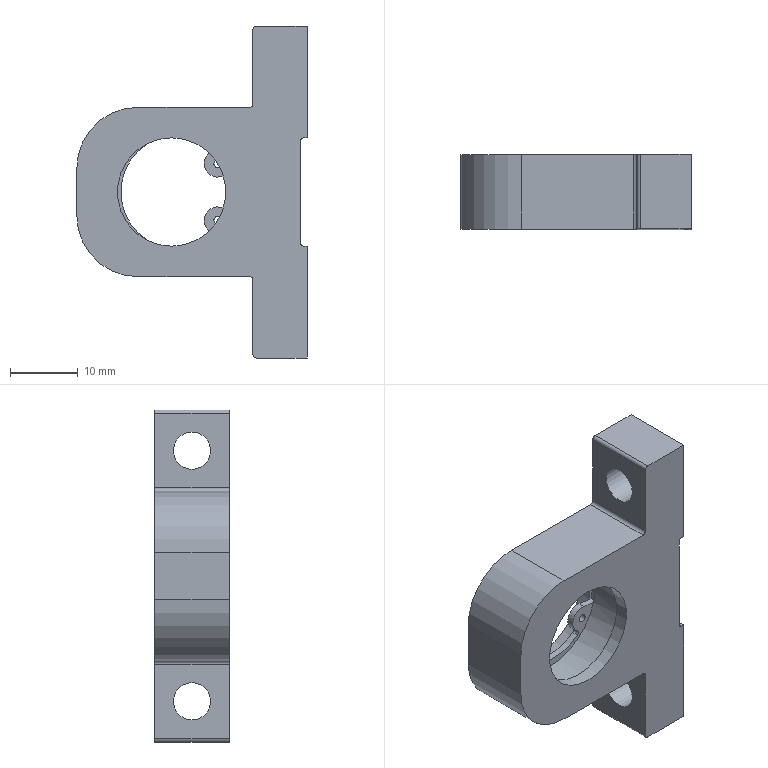Part | NX | features Housing_5003_021_C-BGHA698ZZ-20 2 | 1 solid | 42 faces | box 34 x 11 x 49 mm | volume 7650 mm3 | plane 21 | cylinder 21 | commonest cylinder face diameters 1 x8 1.2 x2 4.006 x2 5.5 x2 18 x2 19 x2
STEP:
#1=CARTESIAN_POINT('',(-207.617,-592.6,-107.974));
#2=VERTEX_POINT('',#1);
#3=CARTESIAN_POINT('',(-207.119,-592.6,-107.9));
#4=VERTEX_POINT('',#3);
#5=CARTESIAN_POINT('',(-209.667,-592.6,-108.281));
#6=DIRECTION('',(0.989,0.,0.1478));
#7=VECTOR('',#6,1000.);
#8=LINE('',#5,#7);
#9=EDGE_CURVE('',#2,#4,#8,.T.);
#10=ORIENTED_EDGE('',*,*,#9,.T.);
#11=CARTESIAN_POINT('',(-207.119,-592.6,-113.1));
#12=VERTEX_POINT('',#11);
#13=CARTESIAN_POINT('',(-216.775,-592.6,-110.5));
#14=DIRECTION('',(0.,-1.,0.));
#15=DIRECTION('',(0.,0.,1.));
#16=AXIS2_PLACEMENT_3D('',#13,#14,#15);
#17=CIRCLE('',#16,10.);
#18=EDGE_CURVE('',#12,#4,#17,.T.);
#19=ORIENTED_EDGE('',*,*,#18,.F.);
#20=CARTESIAN_POINT('',(-207.617,-592.6,-113.026));
#21=VERTEX_POINT('',#20);
#22=CARTESIAN_POINT('',(-209.667,-592.6,-112.719));
#23=DIRECTION('',(-0.989,0.,0.1478));
#24=VECTOR('',#23,1000.);
#25=LINE('',#22,#24);
#26=EDGE_CURVE('',#12,#21,#25,.T.);
#27=ORIENTED_EDGE('',*,*,#26,.T.);
#28=CARTESIAN_POINT('',(-216.775,-592.6,-110.5));
#29=DIRECTION('',(0.,-1.,0.));
#30=DIRECTION('',(0.,0.,1.));
#31=AXIS2_PLACEMENT_3D('',#28,#29,#30);
#32=CIRCLE('',#31,9.5);
#33=EDGE_CURVE('',#21,#2,#32,.T.);
#34=ORIENTED_EDGE('',*,*,#33,.T.);
#35=EDGE_LOOP('',(#10,#19,#27,#34));
#36=FACE_BOUND('',#35,.T.);
#37=CARTESIAN_POINT('',(-226.775,-592.6,-110.5));
#38=DIRECTION('',(0.,-1.,0.));
#39=DIRECTION('',(0.,0.,1.));
#40=AXIS2_PLACEMENT_3D('',#37,#38,#39);
#41=PLANE('',#40);
#42=ADVANCED_FACE('',(#36),#41,.F.);
#43=CARTESIAN_POINT('',(-207.119,-591.6,-107.9));
#44=VERTEX_POINT('',#43);
#45=CARTESIAN_POINT('',(-207.119,-592.6,-107.9));
#46=DIRECTION('',(0.,1.,0.));
#47=VECTOR('',#46,1000.);
#48=LINE('',#45,#47);
#49=EDGE_CURVE('',#4,#44,#48,.T.);
#50=ORIENTED_EDGE('',*,*,#49,.T.);
#51=CARTESIAN_POINT('',(-207.119,-591.6,-113.1));
#52=VERTEX_POINT('',#51);
#53=CARTESIAN_POINT('',(-216.775,-591.6,-110.5));
#54=DIRECTION('',(0.,-1.,0.));
#55=DIRECTION('',(0.,0.,1.));
#56=AXIS2_PLACEMENT_3D('',#53,#54,#55);
#57=CIRCLE('',#56,10.);
#58=EDGE_CURVE('',#52,#44,#57,.T.);
#59=ORIENTED_EDGE('',*,*,#58,.F.);
#60=CARTESIAN_POINT('',(-207.119,-592.6,-113.1));
#61=DIRECTION('',(0.,1.,0.));
#62=VECTOR('',#61,1000.);
#63=LINE('',#60,#62);
#64=EDGE_CURVE('',#12,#52,#63,.T.);
#65=ORIENTED_EDGE('',*,*,#64,.F.);
#66=ORIENTED_EDGE('',*,*,#18,.T.);
#67=EDGE_LOOP('',(#50,#59,#65,#66));
#68=FACE_BOUND('',#67,.T.);
#69=CARTESIAN_POINT('',(-216.775,-600.6,-110.5));
#70=DIRECTION('',(0.,-1.,0.));
#71=DIRECTION('',(0.,0.,1.));
#72=AXIS2_PLACEMENT_3D('',#69,#70,#71);
#73=CYLINDRICAL_SURFACE('',#72,10.);
#74=ADVANCED_FACE('',(#68),#73,.F.);
#75=CARTESIAN_POINT('',(-207.617,-591.6,-107.974));
#76=VERTEX_POINT('',#75);
#77=CARTESIAN_POINT('',(-226.237,-591.6,-110.757));
#78=DIRECTION('',(0.989,0.,0.1478));
#79=VECTOR('',#78,1000.);
#80=LINE('',#77,#79);
#81=EDGE_CURVE('',#76,#44,#80,.T.);
#82=ORIENTED_EDGE('',*,*,#81,.F.);
#83=CARTESIAN_POINT('',(-207.617,-591.6,-113.026));
#84=VERTEX_POINT('',#83);
#85=CARTESIAN_POINT('',(-216.775,-591.6,-110.5));
#86=DIRECTION('',(0.,-1.,0.));
#87=DIRECTION('',(0.,0.,1.));
#88=AXIS2_PLACEMENT_3D('',#85,#86,#87);
#89=CIRCLE('',#88,9.5);
#90=EDGE_CURVE('',#84,#76,#89,.T.);
#91=ORIENTED_EDGE('',*,*,#90,.F.);
#92=CARTESIAN_POINT('',(-209.667,-591.6,-112.719));
#93=DIRECTION('',(-0.989,0.,0.1478));
#94=VECTOR('',#93,1000.);
#95=LINE('',#92,#94);
#96=EDGE_CURVE('',#52,#84,#95,.T.);
#97=ORIENTED_EDGE('',*,*,#96,.F.);
#98=ORIENTED_EDGE('',*,*,#58,.T.);
#99=EDGE_LOOP('',(#82,#91,#97,#98));
#100=FACE_BOUND('',#99,.T.);
#101=CARTESIAN_POINT('',(-226.275,-591.6,-110.5));
#102=DIRECTION('',(0.,1.,0.));
#103=DIRECTION('',(0.,0.,-1.));
#104=AXIS2_PLACEMENT_3D('',#101,#102,#103);
#105=PLANE('',#104);
#106=ADVANCED_FACE('',(#100),#105,.F.);
#107=CARTESIAN_POINT('',(-196.775,-595.1,-126.25));
#108=VERTEX_POINT('',#107);
#109=CARTESIAN_POINT('',(-196.775,-595.1,-129.));
#110=DIRECTION('',(-1.,0.,0.));
#111=DIRECTION('',(0.,0.,1.));
#112=AXIS2_PLACEMENT_3D('',#109,#110,#111);
#113=CIRCLE('',#112,2.75);
#114=EDGE_CURVE('',#108,#108,#113,.T.);
#115=ORIENTED_EDGE('',*,*,#114,.T.);
#116=EDGE_LOOP('',(#115));
#117=FACE_BOUND('',#116,.T.);
#118=CARTESIAN_POINT('',(-196.775,-589.6,-118.5));
#119=VERTEX_POINT('',#118);
#120=CARTESIAN_POINT('',(-196.775,-589.6,-135.));
#121=VERTEX_POINT('',#120);
#122=CARTESIAN_POINT('',(-196.775,-589.6,-135.));
#123=DIRECTION('',(0.,0.,-1.));
#124=VECTOR('',#123,1000.);
#125=LINE('',#122,#124);
#126=EDGE_CURVE('',#119,#121,#125,.T.);
#127=ORIENTED_EDGE('',*,*,#126,.F.);
#128=CARTESIAN_POINT('',(-196.775,-600.6,-118.5));
#129=VERTEX_POINT('',#128);
#130=CARTESIAN_POINT('',(-196.775,-600.6,-118.5));
#131=DIRECTION('',(0.,1.,0.));
#132=VECTOR('',#131,1000.);
#133=LINE('',#130,#132);
#134=EDGE_CURVE('',#129,#119,#133,.T.);
#135=ORIENTED_EDGE('',*,*,#134,.F.);
#136=CARTESIAN_POINT('',(-196.775,-600.6,-135.));
#137=VERTEX_POINT('',#136);
#138=CARTESIAN_POINT('',(-196.775,-600.6,-135.));
#139=DIRECTION('',(0.,0.,-1.));
#140=VECTOR('',#139,1000.);
#141=LINE('',#138,#140);
#142=EDGE_CURVE('',#129,#137,#141,.T.);
#143=ORIENTED_EDGE('',*,*,#142,.T.);
#144=CARTESIAN_POINT('',(-196.775,-600.6,-135.));
#145=DIRECTION('',(0.,1.,0.));
#146=VECTOR('',#145,1000.);
#147=LINE('',#144,#146);
#148=EDGE_CURVE('',#137,#121,#147,.T.);
#149=ORIENTED_EDGE('',*,*,#148,.T.);
#150=EDGE_LOOP('',(#127,#135,#143,#149));
#151=FACE_BOUND('',#150,.T.);
#152=CARTESIAN_POINT('',(-196.775,-600.6,-135.));
#153=DIRECTION('',(1.,0.,0.));
#154=DIRECTION('',(0.,0.,-1.));
#155=AXIS2_PLACEMENT_3D('',#152,#153,#154);
#156=PLANE('',#155);
#157=ADVANCED_FACE('',(#117,#151),#156,.T.);
#158=CARTESIAN_POINT('',(-197.275,-589.6,-118.5));
#159=VERTEX_POINT('',#158);
#160=CARTESIAN_POINT('',(-197.275,-589.6,-118.5));
#161=DIRECTION('',(1.,0.,0.));
#162=VECTOR('',#161,1000.);
#163=LINE('',#160,#162);
#164=EDGE_CURVE('',#159,#119,#163,.T.);
#165=ORIENTED_EDGE('',*,*,#164,.F.);
#166=CARTESIAN_POINT('',(-197.275,-600.6,-118.5));
#167=VERTEX_POINT('',#166);
#168=CARTESIAN_POINT('',(-197.275,-600.6,-118.5));
#169=DIRECTION('',(0.,1.,0.));
#170=VECTOR('',#169,1000.);
#171=LINE('',#168,#170);
#172=EDGE_CURVE('',#167,#159,#171,.T.);
#173=ORIENTED_EDGE('',*,*,#172,.F.);
#174=CARTESIAN_POINT('',(-197.275,-600.6,-118.5));
#175=DIRECTION('',(1.,0.,0.));
#176=VECTOR('',#175,1000.);
#177=LINE('',#174,#176);
#178=EDGE_CURVE('',#167,#129,#177,.T.);
#179=ORIENTED_EDGE('',*,*,#178,.T.);
#180=ORIENTED_EDGE('',*,*,#134,.T.);
#181=EDGE_LOOP('',(#165,#173,#179,#180));
#182=FACE_BOUND('',#181,.T.);
#183=CARTESIAN_POINT('',(-197.275,-600.6,-118.5));
#184=DIRECTION('',(0.,0.,1.));
#185=DIRECTION('',(0.,1.,0.));
#186=AXIS2_PLACEMENT_3D('',#183,#184,#185);
#187=PLANE('',#186);
#188=ADVANCED_FACE('',(#182),#187,.T.);
#189=CARTESIAN_POINT('',(-197.775,-589.6,-118.));
#190=VERTEX_POINT('',#189);
#191=CARTESIAN_POINT('',(-197.275,-589.6,-118.));
#192=DIRECTION('',(0.,-1.,0.));
#193=DIRECTION('',(0.,0.,-1.));
#194=AXIS2_PLACEMENT_3D('',#191,#192,#193);
#195=CIRCLE('',#194,0.5);
#196=EDGE_CURVE('',#190,#159,#195,.T.);
#197=ORIENTED_EDGE('',*,*,#196,.F.);
#198=CARTESIAN_POINT('',(-197.775,-600.6,-118.));
#199=VERTEX_POINT('',#198);
#200=CARTESIAN_POINT('',(-197.775,-600.6,-118.));
#201=DIRECTION('',(0.,1.,0.));
#202=VECTOR('',#201,1000.);
#203=LINE('',#200,#202);
#204=EDGE_CURVE('',#199,#190,#203,.T.);
#205=ORIENTED_EDGE('',*,*,#204,.F.);
#206=CARTESIAN_POINT('',(-197.275,-600.6,-118.));
#207=DIRECTION('',(0.,-1.,0.));
#208=DIRECTION('',(0.,0.,-1.));
#209=AXIS2_PLACEMENT_3D('',#206,#207,#208);
#210=CIRCLE('',#209,0.5);
#211=EDGE_CURVE('',#199,#167,#210,.T.);
#212=ORIENTED_EDGE('',*,*,#211,.T.);
#213=ORIENTED_EDGE('',*,*,#172,.T.);
#214=EDGE_LOOP('',(#197,#205,#212,#213));
#215=FACE_BOUND('',#214,.T.);
#216=CARTESIAN_POINT('',(-197.275,-600.6,-118.));
#217=DIRECTION('',(0.,1.,0.));
#218=DIRECTION('',(0.,0.,-1.));
#219=AXIS2_PLACEMENT_3D('',#216,#217,#218);
#220=CYLINDRICAL_SURFACE('',#219,0.5);
#221=ADVANCED_FACE('',(#215),#220,.F.);
#222=CARTESIAN_POINT('',(-197.775,-589.6,-103.));
#223=VERTEX_POINT('',#222);
#224=CARTESIAN_POINT('',(-197.775,-589.6,-103.));
#225=DIRECTION('',(0.,0.,-1.));
#226=VECTOR('',#225,1000.);
#227=LINE('',#224,#226);
#228=EDGE_CURVE('',#223,#190,#227,.T.);
#229=ORIENTED_EDGE('',*,*,#228,.F.);
#230=CARTESIAN_POINT('',(-197.775,-600.6,-103.));
#231=VERTEX_POINT('',#230);
#232=CARTESIAN_POINT('',(-197.775,-600.6,-103.));
#233=DIRECTION('',(0.,1.,0.));
#234=VECTOR('',#233,1000.);
#235=LINE('',#232,#234);
#236=EDGE_CURVE('',#231,#223,#235,.T.);
#237=ORIENTED_EDGE('',*,*,#236,.F.);
#238=CARTESIAN_POINT('',(-197.775,-600.6,-103.));
#239=DIRECTION('',(0.,0.,-1.));
#240=VECTOR('',#239,1000.);
#241=LINE('',#238,#240);
#242=EDGE_CURVE('',#231,#199,#241,.T.);
#243=ORIENTED_EDGE('',*,*,#242,.T.);
#244=ORIENTED_EDGE('',*,*,#204,.T.);
#245=EDGE_LOOP('',(#229,#237,#243,#244));
#246=FACE_BOUND('',#245,.T.);
#247=CARTESIAN_POINT('',(-197.775,-600.6,-103.));
#248=DIRECTION('',(1.,0.,0.));
#249=DIRECTION('',(0.,0.,-1.));
#250=AXIS2_PLACEMENT_3D('',#247,#248,#249);
#251=PLANE('',#250);
#252=ADVANCED_FACE('',(#246),#251,.T.);
#253=CARTESIAN_POINT('',(-197.275,-589.6,-102.5));
#254=VERTEX_POINT('',#253);
#255=CARTESIAN_POINT('',(-197.275,-589.6,-103.));
#256=DIRECTION('',(0.,-1.,0.));
#257=DIRECTION('',(0.,0.,1.));
#258=AXIS2_PLACEMENT_3D('',#255,#256,#257);
#259=CIRCLE('',#258,0.5);
#260=EDGE_CURVE('',#254,#223,#259,.T.);
#261=ORIENTED_EDGE('',*,*,#260,.F.);
#262=CARTESIAN_POINT('',(-197.275,-600.6,-102.5));
#263=VERTEX_POINT('',#262);
#264=CARTESIAN_POINT('',(-197.275,-600.6,-102.5));
#265=DIRECTION('',(0.,1.,0.));
#266=VECTOR('',#265,1000.);
#267=LINE('',#264,#266);
#268=EDGE_CURVE('',#263,#254,#267,.T.);
#269=ORIENTED_EDGE('',*,*,#268,.F.);
#270=CARTESIAN_POINT('',(-197.275,-600.6,-103.));
#271=DIRECTION('',(0.,-1.,0.));
#272=DIRECTION('',(0.,0.,1.));
#273=AXIS2_PLACEMENT_3D('',#270,#271,#272);
#274=CIRCLE('',#273,0.5);
#275=EDGE_CURVE('',#263,#231,#274,.T.);
#276=ORIENTED_EDGE('',*,*,#275,.T.);
#277=ORIENTED_EDGE('',*,*,#236,.T.);
#278=EDGE_LOOP('',(#261,#269,#276,#277));
#279=FACE_BOUND('',#278,.T.);
#280=CARTESIAN_POINT('',(-197.275,-600.6,-103.));
#281=DIRECTION('',(0.,1.,0.));
#282=DIRECTION('',(0.,0.,-1.));
#283=AXIS2_PLACEMENT_3D('',#280,#281,#282);
#284=CYLINDRICAL_SURFACE('',#283,0.5);
#285=ADVANCED_FACE('',(#279),#284,.F.);
#286=CARTESIAN_POINT('',(-196.775,-589.6,-102.5));
#287=VERTEX_POINT('',#286);
#288=CARTESIAN_POINT('',(-197.275,-589.6,-102.5));
#289=DIRECTION('',(-1.,0.,0.));
#290=VECTOR('',#289,1000.);
#291=LINE('',#288,#290);
#292=EDGE_CURVE('',#287,#254,#291,.T.);
#293=ORIENTED_EDGE('',*,*,#292,.F.);
#294=CARTESIAN_POINT('',(-196.775,-600.6,-102.5));
#295=VERTEX_POINT('',#294);
#296=CARTESIAN_POINT('',(-196.775,-600.6,-102.5));
#297=DIRECTION('',(0.,1.,0.));
#298=VECTOR('',#297,1000.);
#299=LINE('',#296,#298);
#300=EDGE_CURVE('',#295,#287,#299,.T.);
#301=ORIENTED_EDGE('',*,*,#300,.F.);
#302=CARTESIAN_POINT('',(-197.275,-600.6,-102.5));
#303=DIRECTION('',(-1.,0.,0.));
#304=VECTOR('',#303,1000.);
#305=LINE('',#302,#304);
#306=EDGE_CURVE('',#295,#263,#305,.T.);
#307=ORIENTED_EDGE('',*,*,#306,.T.);
#308=ORIENTED_EDGE('',*,*,#268,.T.);
#309=EDGE_LOOP('',(#293,#301,#307,#308));
#310=FACE_BOUND('',#309,.T.);
#311=CARTESIAN_POINT('',(-197.275,-600.6,-102.5));
#312=DIRECTION('',(0.,0.,-1.));
#313=DIRECTION('',(0.,-1.,0.));
#314=AXIS2_PLACEMENT_3D('',#311,#312,#313);
#315=PLANE('',#314);
#316=ADVANCED_FACE('',(#310),#315,.T.);
#317=CARTESIAN_POINT('',(-196.775,-595.1,-89.25));
#318=VERTEX_POINT('',#317);
#319=CARTESIAN_POINT('',(-196.775,-595.1,-92.));
#320=DIRECTION('',(-1.,0.,0.));
#321=DIRECTION('',(0.,0.,1.));
#322=AXIS2_PLACEMENT_3D('',#319,#320,#321);
#323=CIRCLE('',#322,2.75);
#324=EDGE_CURVE('',#318,#318,#323,.T.);
#325=ORIENTED_EDGE('',*,*,#324,.T.);
#326=EDGE_LOOP('',(#325));
#327=FACE_BOUND('',#326,.T.);
#328=CARTESIAN_POINT('',(-196.775,-589.6,-86.));
#329=VERTEX_POINT('',#328);
#330=CARTESIAN_POINT('',(-196.775,-589.6,-102.5));
#331=DIRECTION('',(0.,0.,-1.));
#332=VECTOR('',#331,1000.);
#333=LINE('',#330,#332);
#334=EDGE_CURVE('',#329,#287,#333,.T.);
#335=ORIENTED_EDGE('',*,*,#334,.F.);
#336=CARTESIAN_POINT('',(-196.775,-600.6,-86.));
#337=VERTEX_POINT('',#336);
#338=CARTESIAN_POINT('',(-196.775,-600.6,-86.));
#339=DIRECTION('',(0.,1.,0.));
#340=VECTOR('',#339,1000.);
#341=LINE('',#338,#340);
#342=EDGE_CURVE('',#337,#329,#341,.T.);
#343=ORIENTED_EDGE('',*,*,#342,.F.);
#344=CARTESIAN_POINT('',(-196.775,-600.6,-102.5));
#345=DIRECTION('',(0.,0.,-1.));
#346=VECTOR('',#345,1000.);
#347=LINE('',#344,#346);
#348=EDGE_CURVE('',#337,#295,#347,.T.);
#349=ORIENTED_EDGE('',*,*,#348,.T.);
#350=ORIENTED_EDGE('',*,*,#300,.T.);
#351=EDGE_LOOP('',(#335,#343,#349,#350));
#352=FACE_BOUND('',#351,.T.);
#353=CARTESIAN_POINT('',(-196.775,-600.6,-102.5));
#354=DIRECTION('',(1.,0.,0.));
#355=DIRECTION('',(0.,0.,-1.));
#356=AXIS2_PLACEMENT_3D('',#353,#354,#355);
#357=PLANE('',#356);
#358=ADVANCED_FACE('',(#327,#352),#357,.T.);
#359=CARTESIAN_POINT('',(-204.275,-589.6,-86.));
#360=VERTEX_POINT('',#359);
#361=CARTESIAN_POINT('',(-196.775,-589.6,-86.));
#362=DIRECTION('',(1.,0.,0.));
#363=VECTOR('',#362,1000.);
#364=LINE('',#361,#363);
#365=EDGE_CURVE('',#360,#329,#364,.T.);
#366=ORIENTED_EDGE('',*,*,#365,.F.);
#367=CARTESIAN_POINT('',(-204.275,-600.6,-86.));
#368=VERTEX_POINT('',#367);
#369=CARTESIAN_POINT('',(-204.275,-600.6,-86.));
#370=DIRECTION('',(0.,1.,0.));
#371=VECTOR('',#370,1000.);
#372=LINE('',#369,#371);
#373=EDGE_CURVE('',#368,#360,#372,.T.);
#374=ORIENTED_EDGE('',*,*,#373,.F.);
#375=CARTESIAN_POINT('',(-196.775,-600.6,-86.));
#376=DIRECTION('',(1.,0.,0.));
#377=VECTOR('',#376,1000.);
#378=LINE('',#375,#377);
#379=EDGE_CURVE('',#368,#337,#378,.T.);
#380=ORIENTED_EDGE('',*,*,#379,.T.);
#381=ORIENTED_EDGE('',*,*,#342,.T.);
#382=EDGE_LOOP('',(#366,#374,#380,#381));
#383=FACE_BOUND('',#382,.T.);
#384=CARTESIAN_POINT('',(-196.775,-600.6,-86.));
#385=DIRECTION('',(0.,0.,1.));
#386=DIRECTION('',(0.,1.,0.));
#387=AXIS2_PLACEMENT_3D('',#384,#385,#386);
#388=PLANE('',#387);
#389=ADVANCED_FACE('',(#383),#388,.T.);
#390=CARTESIAN_POINT('',(-204.775,-589.6,-86.5));
#391=VERTEX_POINT('',#390);
#392=CARTESIAN_POINT('',(-204.275,-589.6,-86.5));
#393=DIRECTION('',(0.,1.,0.));
#394=DIRECTION('',(0.,0.,1.));
#395=AXIS2_PLACEMENT_3D('',#392,#393,#394);
#396=CIRCLE('',#395,0.5);
#397=EDGE_CURVE('',#391,#360,#396,.T.);
#398=ORIENTED_EDGE('',*,*,#397,.F.);
#399=CARTESIAN_POINT('',(-204.775,-600.6,-86.5));
#400=VERTEX_POINT('',#399);
#401=CARTESIAN_POINT('',(-204.775,-600.6,-86.5));
#402=DIRECTION('',(0.,1.,0.));
#403=VECTOR('',#402,1000.);
#404=LINE('',#401,#403);
#405=EDGE_CURVE('',#400,#391,#404,.T.);
#406=ORIENTED_EDGE('',*,*,#405,.F.);
#407=CARTESIAN_POINT('',(-204.275,-600.6,-86.5));
#408=DIRECTION('',(0.,1.,0.));
#409=DIRECTION('',(0.,0.,1.));
#410=AXIS2_PLACEMENT_3D('',#407,#408,#409);
#411=CIRCLE('',#410,0.5);
#412=EDGE_CURVE('',#400,#368,#411,.T.);
#413=ORIENTED_EDGE('',*,*,#412,.T.);
#414=ORIENTED_EDGE('',*,*,#373,.T.);
#415=EDGE_LOOP('',(#398,#406,#413,#414));
#416=FACE_BOUND('',#415,.T.);
#417=CARTESIAN_POINT('',(-204.275,-600.6,-86.5));
#418=DIRECTION('',(0.,1.,0.));
#419=DIRECTION('',(0.,0.,-1.));
#420=AXIS2_PLACEMENT_3D('',#417,#418,#419);
#421=CYLINDRICAL_SURFACE('',#420,0.5);
#422=ADVANCED_FACE('',(#416),#421,.T.);
#423=CARTESIAN_POINT('',(-204.775,-595.1,-89.25));
#424=VERTEX_POINT('',#423);
#425=CARTESIAN_POINT('',(-204.775,-595.1,-92.));
#426=DIRECTION('',(-1.,0.,0.));
#427=DIRECTION('',(0.,0.,1.));
#428=AXIS2_PLACEMENT_3D('',#425,#426,#427);
#429=CIRCLE('',#428,2.75);
#430=EDGE_CURVE('',#424,#424,#429,.T.);
#431=ORIENTED_EDGE('',*,*,#430,.F.);
#432=EDGE_LOOP('',(#431));
#433=FACE_BOUND('',#432,.T.);
#434=CARTESIAN_POINT('',(-204.775,-589.6,-97.5));
#435=VERTEX_POINT('',#434);
#436=CARTESIAN_POINT('',(-204.775,-589.6,-86.5));
#437=DIRECTION('',(0.,0.,1.));
#438=VECTOR('',#437,1000.);
#439=LINE('',#436,#438);
#440=EDGE_CURVE('',#435,#391,#439,.T.);
#441=ORIENTED_EDGE('',*,*,#440,.F.);
#442=CARTESIAN_POINT('',(-204.775,-600.6,-97.5));
#443=VERTEX_POINT('',#442);
#444=CARTESIAN_POINT('',(-204.775,-600.6,-97.5));
#445=DIRECTION('',(0.,1.,0.));
#446=VECTOR('',#445,1000.);
#447=LINE('',#444,#446);
#448=EDGE_CURVE('',#443,#435,#447,.T.);
#449=ORIENTED_EDGE('',*,*,#448,.F.);
#450=CARTESIAN_POINT('',(-204.775,-600.6,-86.5));
#451=DIRECTION('',(0.,0.,1.));
#452=VECTOR('',#451,1000.);
#453=LINE('',#450,#452);
#454=EDGE_CURVE('',#443,#400,#453,.T.);
#455=ORIENTED_EDGE('',*,*,#454,.T.);
#456=ORIENTED_EDGE('',*,*,#405,.T.);
#457=EDGE_LOOP('',(#441,#449,#455,#456));
#458=FACE_BOUND('',#457,.T.);
#459=CARTESIAN_POINT('',(-204.775,-600.6,-86.5));
#460=DIRECTION('',(-1.,0.,0.));
#461=DIRECTION('',(0.,0.,1.));
#462=AXIS2_PLACEMENT_3D('',#459,#460,#461);
#463=PLANE('',#462);
#464=ADVANCED_FACE('',(#433,#458),#463,.T.);
#465=CARTESIAN_POINT('',(-205.275,-589.6,-98.));
#466=VERTEX_POINT('',#465);
#467=CARTESIAN_POINT('',(-205.275,-589.6,-97.5));
#468=DIRECTION('',(0.,-1.,0.));
#469=DIRECTION('',(0.,0.,1.));
#470=AXIS2_PLACEMENT_3D('',#467,#468,#469);
#471=CIRCLE('',#470,0.5);
#472=EDGE_CURVE('',#466,#435,#471,.T.);
#473=ORIENTED_EDGE('',*,*,#472,.F.);
#474=CARTESIAN_POINT('',(-205.275,-600.6,-98.));
#475=VERTEX_POINT('',#474);
#476=CARTESIAN_POINT('',(-205.275,-600.6,-98.));
#477=DIRECTION('',(0.,1.,0.));
#478=VECTOR('',#477,1000.);
#479=LINE('',#476,#478);
#480=EDGE_CURVE('',#475,#466,#479,.T.);
#481=ORIENTED_EDGE('',*,*,#480,.F.);
#482=CARTESIAN_POINT('',(-205.275,-600.6,-97.5));
#483=DIRECTION('',(0.,-1.,0.));
#484=DIRECTION('',(0.,0.,1.));
#485=AXIS2_PLACEMENT_3D('',#482,#483,#484);
#486=CIRCLE('',#485,0.5);
#487=EDGE_CURVE('',#475,#443,#486,.T.);
#488=ORIENTED_EDGE('',*,*,#487,.T.);
#489=ORIENTED_EDGE('',*,*,#448,.T.);
#490=EDGE_LOOP('',(#473,#481,#488,#489));
#491=FACE_BOUND('',#490,.T.);
#492=CARTESIAN_POINT('',(-205.275,-600.6,-97.5));
#493=DIRECTION('',(0.,1.,0.));
#494=DIRECTION('',(0.,0.,-1.));
#495=AXIS2_PLACEMENT_3D('',#492,#493,#494);
#496=CYLINDRICAL_SURFACE('',#495,0.5);
#497=ADVANCED_FACE('',(#491),#496,.F.);
#498=CARTESIAN_POINT('',(-221.775,-589.6,-98.));
#499=VERTEX_POINT('',#498);
#500=CARTESIAN_POINT('',(-205.275,-589.6,-98.));
#501=DIRECTION('',(1.,0.,0.));
#502=VECTOR('',#501,1000.);
#503=LINE('',#500,#502);
#504=EDGE_CURVE('',#499,#466,#503,.T.);
#505=ORIENTED_EDGE('',*,*,#504,.F.);
#506=CARTESIAN_POINT('',(-221.775,-600.6,-98.));
#507=VERTEX_POINT('',#506);
#508=CARTESIAN_POINT('',(-221.775,-600.6,-98.));
#509=DIRECTION('',(0.,1.,0.));
#510=VECTOR('',#509,1000.);
#511=LINE('',#508,#510);
#512=EDGE_CURVE('',#507,#499,#511,.T.);
#513=ORIENTED_EDGE('',*,*,#512,.F.);
#514=CARTESIAN_POINT('',(-205.275,-600.6,-98.));
#515=DIRECTION('',(1.,0.,0.));
#516=VECTOR('',#515,1000.);
#517=LINE('',#514,#516);
#518=EDGE_CURVE('',#507,#475,#517,.T.);
#519=ORIENTED_EDGE('',*,*,#518,.T.);
#520=ORIENTED_EDGE('',*,*,#480,.T.);
#521=EDGE_LOOP('',(#505,#513,#519,#520));
#522=FACE_BOUND('',#521,.T.);
#523=CARTESIAN_POINT('',(-205.275,-600.6,-98.));
#524=DIRECTION('',(0.,0.,1.));
#525=DIRECTION('',(1.,0.,0.));
#526=AXIS2_PLACEMENT_3D('',#523,#524,#525);
#527=PLANE('',#526);
#528=ADVANCED_FACE('',(#522),#527,.T.);
#529=CARTESIAN_POINT('',(-230.775,-589.6,-107.));
#530=VERTEX_POINT('',#529);
#531=CARTESIAN_POINT('',(-221.775,-589.6,-107.));
#532=DIRECTION('',(0.,1.,0.));
#533=DIRECTION('',(0.,0.,1.));
#534=AXIS2_PLACEMENT_3D('',#531,#532,#533);
#535=CIRCLE('',#534,9.);
#536=EDGE_CURVE('',#530,#499,#535,.T.);
#537=ORIENTED_EDGE('',*,*,#536,.F.);
#538=CARTESIAN_POINT('',(-230.775,-600.6,-107.));
#539=VERTEX_POINT('',#538);
#540=CARTESIAN_POINT('',(-230.775,-600.6,-107.));
#541=DIRECTION('',(0.,1.,0.));
#542=VECTOR('',#541,1000.);
#543=LINE('',#540,#542);
#544=EDGE_CURVE('',#539,#530,#543,.T.);
#545=ORIENTED_EDGE('',*,*,#544,.F.);
#546=CARTESIAN_POINT('',(-221.775,-600.6,-107.));
#547=DIRECTION('',(0.,1.,0.));
#548=DIRECTION('',(0.,0.,1.));
#549=AXIS2_PLACEMENT_3D('',#546,#547,#548);
#550=CIRCLE('',#549,9.);
#551=EDGE_CURVE('',#539,#507,#550,.T.);
#552=ORIENTED_EDGE('',*,*,#551,.T.);
#553=ORIENTED_EDGE('',*,*,#512,.T.);
#554=EDGE_LOOP('',(#537,#545,#552,#553));
#555=FACE_BOUND('',#554,.T.);
#556=CARTESIAN_POINT('',(-221.775,-600.6,-107.));
#557=DIRECTION('',(0.,1.,0.));
#558=DIRECTION('',(0.,0.,-1.));
#559=AXIS2_PLACEMENT_3D('',#556,#557,#558);
#560=CYLINDRICAL_SURFACE('',#559,9.);
#561=ADVANCED_FACE('',(#555),#560,.T.);
#562=CARTESIAN_POINT('',(-230.775,-589.6,-114.));
#563=VERTEX_POINT('',#562);
#564=CARTESIAN_POINT('',(-230.775,-589.6,-107.));
#565=DIRECTION('',(0.,0.,1.));
#566=VECTOR('',#565,1000.);
#567=LINE('',#564,#566);
#568=EDGE_CURVE('',#563,#530,#567,.T.);
#569=ORIENTED_EDGE('',*,*,#568,.F.);
#570=CARTESIAN_POINT('',(-230.775,-600.6,-114.));
#571=VERTEX_POINT('',#570);
#572=CARTESIAN_POINT('',(-230.775,-600.6,-114.));
#573=DIRECTION('',(0.,1.,0.));
#574=VECTOR('',#573,1000.);
#575=LINE('',#572,#574);
#576=EDGE_CURVE('',#571,#563,#575,.T.);
#577=ORIENTED_EDGE('',*,*,#576,.F.);
#578=CARTESIAN_POINT('',(-230.775,-600.6,-107.));
#579=DIRECTION('',(0.,0.,1.));
#580=VECTOR('',#579,1000.);
#581=LINE('',#578,#580);
#582=EDGE_CURVE('',#571,#539,#581,.T.);
#583=ORIENTED_EDGE('',*,*,#582,.T.);
#584=ORIENTED_EDGE('',*,*,#544,.T.);
#585=EDGE_LOOP('',(#569,#577,#583,#584));
#586=FACE_BOUND('',#585,.T.);
#587=CARTESIAN_POINT('',(-230.775,-600.6,-107.));
#588=DIRECTION('',(-1.,0.,0.));
#589=DIRECTION('',(0.,0.,1.));
#590=AXIS2_PLACEMENT_3D('',#587,#588,#589);
#591=PLANE('',#590);
#592=ADVANCED_FACE('',(#586),#591,.T.);
#593=CARTESIAN_POINT('',(-221.775,-589.6,-123.));
#594=VERTEX_POINT('',#593);
#595=CARTESIAN_POINT('',(-221.775,-589.6,-114.));
#596=DIRECTION('',(0.,1.,0.));
#597=DIRECTION('',(0.,0.,-1.));
#598=AXIS2_PLACEMENT_3D('',#595,#596,#597);
#599=CIRCLE('',#598,9.);
#600=EDGE_CURVE('',#594,#563,#599,.T.);
#601=ORIENTED_EDGE('',*,*,#600,.F.);
#602=CARTESIAN_POINT('',(-221.775,-600.6,-123.));
#603=VERTEX_POINT('',#602);
#604=CARTESIAN_POINT('',(-221.775,-600.6,-123.));
#605=DIRECTION('',(0.,1.,0.));
#606=VECTOR('',#605,1000.);
#607=LINE('',#604,#606);
#608=EDGE_CURVE('',#603,#594,#607,.T.);
#609=ORIENTED_EDGE('',*,*,#608,.F.);
#610=CARTESIAN_POINT('',(-221.775,-600.6,-114.));
#611=DIRECTION('',(0.,1.,0.));
#612=DIRECTION('',(0.,0.,-1.));
#613=AXIS2_PLACEMENT_3D('',#610,#611,#612);
#614=CIRCLE('',#613,9.);
#615=EDGE_CURVE('',#603,#571,#614,.T.);
#616=ORIENTED_EDGE('',*,*,#615,.T.);
#617=ORIENTED_EDGE('',*,*,#576,.T.);
#618=EDGE_LOOP('',(#601,#609,#616,#617));
#619=FACE_BOUND('',#618,.T.);
#620=CARTESIAN_POINT('',(-221.775,-600.6,-114.));
#621=DIRECTION('',(0.,1.,0.));
#622=DIRECTION('',(0.,0.,-1.));
#623=AXIS2_PLACEMENT_3D('',#620,#621,#622);
#624=CYLINDRICAL_SURFACE('',#623,9.);
#625=ADVANCED_FACE('',(#619),#624,.T.);
#626=CARTESIAN_POINT('',(-205.275,-589.6,-123.));
#627=VERTEX_POINT('',#626);
#628=CARTESIAN_POINT('',(-221.775,-589.6,-123.));
#629=DIRECTION('',(-1.,0.,0.));
#630=VECTOR('',#629,1000.);
#631=LINE('',#628,#630);
#632=EDGE_CURVE('',#627,#594,#631,.T.);
#633=ORIENTED_EDGE('',*,*,#632,.F.);
#634=CARTESIAN_POINT('',(-205.275,-600.6,-123.));
#635=VERTEX_POINT('',#634);
#636=CARTESIAN_POINT('',(-205.275,-600.6,-123.));
#637=DIRECTION('',(0.,1.,0.));
#638=VECTOR('',#637,1000.);
#639=LINE('',#636,#638);
#640=EDGE_CURVE('',#635,#627,#639,.T.);
#641=ORIENTED_EDGE('',*,*,#640,.F.);
#642=CARTESIAN_POINT('',(-221.775,-600.6,-123.));
#643=DIRECTION('',(-1.,0.,0.));
#644=VECTOR('',#643,1000.);
#645=LINE('',#642,#644);
#646=EDGE_CURVE('',#635,#603,#645,.T.);
#647=ORIENTED_EDGE('',*,*,#646,.T.);
#648=ORIENTED_EDGE('',*,*,#608,.T.);
#649=EDGE_LOOP('',(#633,#641,#647,#648));
#650=FACE_BOUND('',#649,.T.);
#651=CARTESIAN_POINT('',(-221.775,-600.6,-123.));
#652=DIRECTION('',(0.,0.,-1.));
#653=DIRECTION('',(-1.,0.,0.));
#654=AXIS2_PLACEMENT_3D('',#651,#652,#653);
#655=PLANE('',#654);
#656=ADVANCED_FACE('',(#650),#655,.T.);
#657=CARTESIAN_POINT('',(-204.775,-589.6,-123.5));
#658=VERTEX_POINT('',#657);
#659=CARTESIAN_POINT('',(-205.275,-589.6,-123.5));
#660=DIRECTION('',(0.,-1.,0.));
#661=DIRECTION('',(0.,0.,1.));
#662=AXIS2_PLACEMENT_3D('',#659,#660,#661);
#663=CIRCLE('',#662,0.5);
#664=EDGE_CURVE('',#658,#627,#663,.T.);
#665=ORIENTED_EDGE('',*,*,#664,.F.);
#666=CARTESIAN_POINT('',(-204.775,-600.6,-123.5));
#667=VERTEX_POINT('',#666);
#668=CARTESIAN_POINT('',(-204.775,-600.6,-123.5));
#669=DIRECTION('',(0.,1.,0.));
#670=VECTOR('',#669,1000.);
#671=LINE('',#668,#670);
#672=EDGE_CURVE('',#667,#658,#671,.T.);
#673=ORIENTED_EDGE('',*,*,#672,.F.);
#674=CARTESIAN_POINT('',(-205.275,-600.6,-123.5));
#675=DIRECTION('',(0.,-1.,0.));
#676=DIRECTION('',(0.,0.,1.));
#677=AXIS2_PLACEMENT_3D('',#674,#675,#676);
#678=CIRCLE('',#677,0.5);
#679=EDGE_CURVE('',#667,#635,#678,.T.);
#680=ORIENTED_EDGE('',*,*,#679,.T.);
#681=ORIENTED_EDGE('',*,*,#640,.T.);
#682=EDGE_LOOP('',(#665,#673,#680,#681));
#683=FACE_BOUND('',#682,.T.);
#684=CARTESIAN_POINT('',(-205.275,-600.6,-123.5));
#685=DIRECTION('',(0.,1.,0.));
#686=DIRECTION('',(0.,0.,-1.));
#687=AXIS2_PLACEMENT_3D('',#684,#685,#686);
#688=CYLINDRICAL_SURFACE('',#687,0.5);
#689=ADVANCED_FACE('',(#683),#688,.F.);
#690=CARTESIAN_POINT('',(-204.775,-595.1,-126.25));
#691=VERTEX_POINT('',#690);
#692=CARTESIAN_POINT('',(-204.775,-595.1,-129.));
#693=DIRECTION('',(-1.,0.,0.));
#694=DIRECTION('',(0.,0.,1.));
#695=AXIS2_PLACEMENT_3D('',#692,#693,#694);
#696=CIRCLE('',#695,2.75);
#697=EDGE_CURVE('',#691,#691,#696,.T.);
#698=ORIENTED_EDGE('',*,*,#697,.F.);
#699=EDGE_LOOP('',(#698));
#700=FACE_BOUND('',#699,.T.);
#701=CARTESIAN_POINT('',(-204.775,-589.6,-134.5));
#702=VERTEX_POINT('',#701);
#703=CARTESIAN_POINT('',(-204.775,-589.6,-123.5));
#704=DIRECTION('',(0.,0.,1.));
#705=VECTOR('',#704,1000.);
#706=LINE('',#703,#705);
#707=EDGE_CURVE('',#702,#658,#706,.T.);
#708=ORIENTED_EDGE('',*,*,#707,.F.);
#709=CARTESIAN_POINT('',(-204.775,-600.6,-134.5));
#710=VERTEX_POINT('',#709);
#711=CARTESIAN_POINT('',(-204.775,-600.6,-134.5));
#712=DIRECTION('',(0.,1.,0.));
#713=VECTOR('',#712,1000.);
#714=LINE('',#711,#713);
#715=EDGE_CURVE('',#710,#702,#714,.T.);
#716=ORIENTED_EDGE('',*,*,#715,.F.);
#717=CARTESIAN_POINT('',(-204.775,-600.6,-123.5));
#718=DIRECTION('',(0.,0.,1.));
#719=VECTOR('',#718,1000.);
#720=LINE('',#717,#719);
#721=EDGE_CURVE('',#710,#667,#720,.T.);
#722=ORIENTED_EDGE('',*,*,#721,.T.);
#723=ORIENTED_EDGE('',*,*,#672,.T.);
#724=EDGE_LOOP('',(#708,#716,#722,#723));
#725=FACE_BOUND('',#724,.T.);
#726=CARTESIAN_POINT('',(-204.775,-600.6,-123.5));
#727=DIRECTION('',(-1.,0.,0.));
#728=DIRECTION('',(0.,0.,1.));
#729=AXIS2_PLACEMENT_3D('',#726,#727,#728);
#730=PLANE('',#729);
#731=ADVANCED_FACE('',(#700,#725),#730,.T.);
#732=CARTESIAN_POINT('',(-204.275,-589.6,-135.));
#733=VERTEX_POINT('',#732);
#734=CARTESIAN_POINT('',(-204.275,-589.6,-134.5));
#735=DIRECTION('',(0.,1.,0.));
#736=DIRECTION('',(0.,0.,-1.));
#737=AXIS2_PLACEMENT_3D('',#734,#735,#736);
#738=CIRCLE('',#737,0.5);
#739=EDGE_CURVE('',#733,#702,#738,.T.);
#740=ORIENTED_EDGE('',*,*,#739,.F.);
#741=CARTESIAN_POINT('',(-204.275,-600.6,-135.));
#742=VERTEX_POINT('',#741);
#743=CARTESIAN_POINT('',(-204.275,-600.6,-135.));
#744=DIRECTION('',(0.,1.,0.));
#745=VECTOR('',#744,1000.);
#746=LINE('',#743,#745);
#747=EDGE_CURVE('',#742,#733,#746,.T.);
#748=ORIENTED_EDGE('',*,*,#747,.F.);
#749=CARTESIAN_POINT('',(-204.275,-600.6,-134.5));
#750=DIRECTION('',(0.,1.,0.));
#751=DIRECTION('',(0.,0.,-1.));
#752=AXIS2_PLACEMENT_3D('',#749,#750,#751);
#753=CIRCLE('',#752,0.5);
#754=EDGE_CURVE('',#742,#710,#753,.T.);
#755=ORIENTED_EDGE('',*,*,#754,.T.);
#756=ORIENTED_EDGE('',*,*,#715,.T.);
#757=EDGE_LOOP('',(#740,#748,#755,#756));
#758=FACE_BOUND('',#757,.T.);
#759=CARTESIAN_POINT('',(-204.275,-600.6,-134.5));
#760=DIRECTION('',(0.,1.,0.));
#761=DIRECTION('',(0.,0.,-1.));
#762=AXIS2_PLACEMENT_3D('',#759,#760,#761);
#763=CYLINDRICAL_SURFACE('',#762,0.5);
#764=ADVANCED_FACE('',(#758),#763,.T.);
#765=CARTESIAN_POINT('',(-204.275,-589.6,-135.));
#766=DIRECTION('',(-1.,0.,0.));
#767=VECTOR('',#766,1000.);
#768=LINE('',#765,#767);
#769=EDGE_CURVE('',#121,#733,#768,.T.);
#770=ORIENTED_EDGE('',*,*,#769,.F.);
#771=ORIENTED_EDGE('',*,*,#148,.F.);
#772=CARTESIAN_POINT('',(-204.275,-600.6,-135.));
#773=DIRECTION('',(-1.,0.,0.));
#774=VECTOR('',#773,1000.);
#775=LINE('',#772,#774);
#776=EDGE_CURVE('',#137,#742,#775,.T.);
#777=ORIENTED_EDGE('',*,*,#776,.T.);
#778=ORIENTED_EDGE('',*,*,#747,.T.);
#779=EDGE_LOOP('',(#770,#771,#777,#778));
#780=FACE_BOUND('',#779,.T.);
#781=CARTESIAN_POINT('',(-204.275,-600.6,-135.));
#782=DIRECTION('',(0.,0.,-1.));
#783=DIRECTION('',(0.,-1.,0.));
#784=AXIS2_PLACEMENT_3D('',#781,#782,#783);
#785=PLANE('',#784);
#786=ADVANCED_FACE('',(#780),#785,.T.);
#787=CARTESIAN_POINT('',(-216.775,-600.6,-102.5));
#788=VERTEX_POINT('',#787);
#789=CARTESIAN_POINT('',(-216.775,-600.6,-110.5));
#790=DIRECTION('',(0.,-1.,0.));
#791=DIRECTION('',(0.,0.,1.));
#792=AXIS2_PLACEMENT_3D('',#789,#790,#791);
#793=CIRCLE('',#792,8.);
#794=EDGE_CURVE('',#788,#788,#793,.T.);
#795=ORIENTED_EDGE('',*,*,#794,.F.);
#796=EDGE_LOOP('',(#795));
#797=FACE_BOUND('',#796,.T.);
#798=ORIENTED_EDGE('',*,*,#142,.F.);
#799=ORIENTED_EDGE('',*,*,#178,.F.);
#800=ORIENTED_EDGE('',*,*,#211,.F.);
#801=ORIENTED_EDGE('',*,*,#242,.F.);
#802=ORIENTED_EDGE('',*,*,#275,.F.);
#803=ORIENTED_EDGE('',*,*,#306,.F.);
#804=ORIENTED_EDGE('',*,*,#348,.F.);
#805=ORIENTED_EDGE('',*,*,#379,.F.);
#806=ORIENTED_EDGE('',*,*,#412,.F.);
#807=ORIENTED_EDGE('',*,*,#454,.F.);
#808=ORIENTED_EDGE('',*,*,#487,.F.);
#809=ORIENTED_EDGE('',*,*,#518,.F.);
#810=ORIENTED_EDGE('',*,*,#551,.F.);
#811=ORIENTED_EDGE('',*,*,#582,.F.);
#812=ORIENTED_EDGE('',*,*,#615,.F.);
#813=ORIENTED_EDGE('',*,*,#646,.F.);
#814=ORIENTED_EDGE('',*,*,#679,.F.);
#815=ORIENTED_EDGE('',*,*,#721,.F.);
#816=ORIENTED_EDGE('',*,*,#754,.F.);
#817=ORIENTED_EDGE('',*,*,#776,.F.);
#818=EDGE_LOOP('',(#798,#799,#800,#801,#802,#803,#804,#805,#806,#807,#808,#809,#810,#811,#812,#813,#814,#815,#816,#817));
#819=FACE_BOUND('',#818,.T.);
#820=CARTESIAN_POINT('',(-197.275,-600.6,-118.));
#821=DIRECTION('',(0.,1.,0.));
#822=DIRECTION('',(0.,0.,-1.));
#823=AXIS2_PLACEMENT_3D('',#820,#821,#822);
#824=PLANE('',#823);
#825=ADVANCED_FACE('',(#797,#819),#824,.F.);
#826=CARTESIAN_POINT('',(-216.775,-589.6,-101.));
#827=VERTEX_POINT('',#826);
#828=CARTESIAN_POINT('',(-216.775,-589.6,-110.5));
#829=DIRECTION('',(0.,-1.,0.));
#830=DIRECTION('',(0.,0.,1.));
#831=AXIS2_PLACEMENT_3D('',#828,#829,#830);
#832=CIRCLE('',#831,9.5);
#833=EDGE_CURVE('',#827,#827,#832,.T.);
#834=ORIENTED_EDGE('',*,*,#833,.T.);
#835=EDGE_LOOP('',(#834));
#836=FACE_BOUND('',#835,.T.);
#837=ORIENTED_EDGE('',*,*,#126,.T.);
#838=ORIENTED_EDGE('',*,*,#769,.T.);
#839=ORIENTED_EDGE('',*,*,#739,.T.);
#840=ORIENTED_EDGE('',*,*,#707,.T.);
#841=ORIENTED_EDGE('',*,*,#664,.T.);
#842=ORIENTED_EDGE('',*,*,#632,.T.);
#843=ORIENTED_EDGE('',*,*,#600,.T.);
#844=ORIENTED_EDGE('',*,*,#568,.T.);
#845=ORIENTED_EDGE('',*,*,#536,.T.);
#846=ORIENTED_EDGE('',*,*,#504,.T.);
#847=ORIENTED_EDGE('',*,*,#472,.T.);
#848=ORIENTED_EDGE('',*,*,#440,.T.);
#849=ORIENTED_EDGE('',*,*,#397,.T.);
#850=ORIENTED_EDGE('',*,*,#365,.T.);
#851=ORIENTED_EDGE('',*,*,#334,.T.);
#852=ORIENTED_EDGE('',*,*,#292,.T.);
#853=ORIENTED_EDGE('',*,*,#260,.T.);
#854=ORIENTED_EDGE('',*,*,#228,.T.);
#855=ORIENTED_EDGE('',*,*,#196,.T.);
#856=ORIENTED_EDGE('',*,*,#164,.T.);
#857=EDGE_LOOP('',(#837,#838,#839,#840,#841,#842,#843,#844,#845,#846,#847,#848,#849,#850,#851,#852,#853,#854,#855,#856));
#858=FACE_BOUND('',#857,.T.);
#859=CARTESIAN_POINT('',(-197.275,-589.6,-118.));
#860=DIRECTION('',(0.,1.,0.));
#861=DIRECTION('',(0.,0.,-1.));
#862=AXIS2_PLACEMENT_3D('',#859,#860,#861);
#863=PLANE('',#862);
#864=ADVANCED_FACE('',(#836,#858),#863,.T.);
#865=ORIENTED_EDGE('',*,*,#833,.F.);
#866=EDGE_LOOP('',(#865));
#867=FACE_BOUND('',#866,.T.);
#868=ORIENTED_EDGE('',*,*,#90,.T.);
#869=CARTESIAN_POINT('',(-216.775,-591.6,-110.5));
#870=DIRECTION('',(0.,-1.,0.));
#871=DIRECTION('',(0.,0.,1.));
#872=AXIS2_PLACEMENT_3D('',#869,#870,#871);
#873=CIRCLE('',#872,9.5);
#874=EDGE_CURVE('',#76,#84,#873,.T.);
#875=ORIENTED_EDGE('',*,*,#874,.T.);
#876=EDGE_LOOP('',(#868,#875));
#877=FACE_BOUND('',#876,.T.);
#878=CARTESIAN_POINT('',(-216.775,-600.6,-110.5));
#879=DIRECTION('',(0.,-1.,0.));
#880=DIRECTION('',(0.,0.,1.));
#881=AXIS2_PLACEMENT_3D('',#878,#879,#880);
#882=CYLINDRICAL_SURFACE('',#881,9.5);
#883=ADVANCED_FACE('',(#867,#877),#882,.F.);
#884=CARTESIAN_POINT('',(-216.775,-598.6,-102.5));
#885=VERTEX_POINT('',#884);
#886=CARTESIAN_POINT('',(-216.775,-598.6,-110.5));
#887=DIRECTION('',(0.,-1.,0.));
#888=DIRECTION('',(0.,0.,1.));
#889=AXIS2_PLACEMENT_3D('',#886,#887,#888);
#890=CIRCLE('',#889,8.);
#891=EDGE_CURVE('',#885,#885,#890,.T.);
#892=ORIENTED_EDGE('',*,*,#891,.F.);
#893=EDGE_LOOP('',(#892));
#894=FACE_BOUND('',#893,.T.);
#895=ORIENTED_EDGE('',*,*,#794,.T.);
#896=EDGE_LOOP('',(#895));
#897=FACE_BOUND('',#896,.T.);
#898=CARTESIAN_POINT('',(-216.775,-600.6,-110.5));
#899=DIRECTION('',(0.,-1.,0.));
#900=DIRECTION('',(0.,0.,1.));
#901=AXIS2_PLACEMENT_3D('',#898,#899,#900);
#902=CYLINDRICAL_SURFACE('',#901,8.);
#903=ADVANCED_FACE('',(#894,#897),#902,.F.);
#904=CARTESIAN_POINT('',(-216.775,-598.6,-101.));
#905=VERTEX_POINT('',#904);
#906=CARTESIAN_POINT('',(-216.775,-598.6,-110.5));
#907=DIRECTION('',(0.,-1.,0.));
#908=DIRECTION('',(0.,0.,1.));
#909=AXIS2_PLACEMENT_3D('',#906,#907,#908);
#910=CIRCLE('',#909,9.5);
#911=EDGE_CURVE('',#905,#905,#910,.T.);
#912=ORIENTED_EDGE('',*,*,#911,.F.);
#913=EDGE_LOOP('',(#912));
#914=FACE_BOUND('',#913,.T.);
#915=ORIENTED_EDGE('',*,*,#891,.T.);
#916=EDGE_LOOP('',(#915));
#917=FACE_BOUND('',#916,.T.);
#918=CARTESIAN_POINT('',(-226.275,-598.6,-110.5));
#919=DIRECTION('',(0.,-1.,0.));
#920=DIRECTION('',(0.,0.,1.));
#921=AXIS2_PLACEMENT_3D('',#918,#919,#920);
#922=PLANE('',#921);
#923=ADVANCED_FACE('',(#914,#917),#922,.F.);
#924=ORIENTED_EDGE('',*,*,#33,.F.);
#925=CARTESIAN_POINT('',(-216.775,-592.6,-110.5));
#926=DIRECTION('',(0.,-1.,0.));
#927=DIRECTION('',(0.,0.,1.));
#928=AXIS2_PLACEMENT_3D('',#925,#926,#927);
#929=CIRCLE('',#928,9.5);
#930=EDGE_CURVE('',#21,#2,#929,.F.);
#931=ORIENTED_EDGE('',*,*,#930,.T.);
#932=EDGE_LOOP('',(#924,#931));
#933=FACE_BOUND('',#932,.T.);
#934=ORIENTED_EDGE('',*,*,#911,.T.);
#935=EDGE_LOOP('',(#934));
#936=FACE_BOUND('',#935,.T.);
#937=CARTESIAN_POINT('',(-216.775,-600.6,-110.5));
#938=DIRECTION('',(0.,-1.,0.));
#939=DIRECTION('',(0.,0.,1.));
#940=AXIS2_PLACEMENT_3D('',#937,#938,#939);
#941=CYLINDRICAL_SURFACE('',#940,9.5);
#942=ADVANCED_FACE('',(#933,#936),#941,.F.);
#943=ORIENTED_EDGE('',*,*,#324,.F.);
#944=EDGE_LOOP('',(#943));
#945=FACE_BOUND('',#944,.T.);
#946=ORIENTED_EDGE('',*,*,#430,.T.);
#947=EDGE_LOOP('',(#946));
#948=FACE_BOUND('',#947,.T.);
#949=CARTESIAN_POINT('',(-204.775,-595.1,-92.));
#950=DIRECTION('',(-1.,0.,0.));
#951=DIRECTION('',(0.,0.,1.));
#952=AXIS2_PLACEMENT_3D('',#949,#950,#951);
#953=CYLINDRICAL_SURFACE('',#952,2.75);
#954=ADVANCED_FACE('',(#945,#948),#953,.F.);
#955=ORIENTED_EDGE('',*,*,#114,.F.);
#956=EDGE_LOOP('',(#955));
#957=FACE_BOUND('',#956,.T.);
#958=ORIENTED_EDGE('',*,*,#697,.T.);
#959=EDGE_LOOP('',(#958));
#960=FACE_BOUND('',#959,.T.);
#961=CARTESIAN_POINT('',(-204.775,-595.1,-129.));
#962=DIRECTION('',(-1.,0.,0.));
#963=DIRECTION('',(0.,0.,1.));
#964=AXIS2_PLACEMENT_3D('',#961,#962,#963);
#965=CYLINDRICAL_SURFACE('',#964,2.75);
#966=ADVANCED_FACE('',(#957,#960),#965,.F.);
#967=CARTESIAN_POINT('',(-209.963,-592.6,-105.7));
#968=VERTEX_POINT('',#967);
#969=CARTESIAN_POINT('',(-209.963,-592.6,-106.3));
#970=DIRECTION('',(0.,-1.,0.));
#971=DIRECTION('',(0.,0.,1.));
#972=AXIS2_PLACEMENT_3D('',#969,#970,#971);
#973=CIRCLE('',#972,0.6);
#974=EDGE_CURVE('',#968,#968,#973,.T.);
#975=ORIENTED_EDGE('',*,*,#974,.F.);
#976=EDGE_LOOP('',(#975));
#977=FACE_BOUND('',#976,.T.);
#978=CARTESIAN_POINT('',(-209.963,-592.6,-114.1));
#979=VERTEX_POINT('',#978);
#980=CARTESIAN_POINT('',(-209.963,-592.6,-114.7));
#981=DIRECTION('',(0.,-1.,0.));
#982=DIRECTION('',(0.,0.,1.));
#983=AXIS2_PLACEMENT_3D('',#980,#981,#982);
#984=CIRCLE('',#983,0.6);
#985=EDGE_CURVE('',#979,#979,#984,.T.);
#986=ORIENTED_EDGE('',*,*,#985,.F.);
#987=EDGE_LOOP('',(#986));
#988=FACE_BOUND('',#987,.T.);
#989=ORIENTED_EDGE('',*,*,#930,.F.);
#990=CARTESIAN_POINT('',(-209.667,-592.6,-112.719));
#991=VERTEX_POINT('',#990);
#992=CARTESIAN_POINT('',(-209.667,-592.6,-112.719));
#993=DIRECTION('',(-0.989,0.,0.1478));
#994=VECTOR('',#993,1000.);
#995=LINE('',#992,#994);
#996=EDGE_CURVE('',#21,#991,#995,.T.);
#997=ORIENTED_EDGE('',*,*,#996,.T.);
#998=CARTESIAN_POINT('',(-210.987,-592.6,-116.421));
#999=VERTEX_POINT('',#998);
#1000=CARTESIAN_POINT('',(-209.963,-592.6,-114.7));
#1001=DIRECTION('',(0.,-1.,0.));
#1002=DIRECTION('',(0.,0.,1.));
#1003=AXIS2_PLACEMENT_3D('',#1000,#1001,#1002);
#1004=CIRCLE('',#1003,2.003);
#1005=EDGE_CURVE('',#991,#999,#1004,.T.);
#1006=ORIENTED_EDGE('',*,*,#1005,.T.);
#1007=CARTESIAN_POINT('',(-210.947,-592.6,-117.254));
#1008=VERTEX_POINT('',#1007);
#1009=CARTESIAN_POINT('',(-211.243,-592.6,-116.851));
#1010=DIRECTION('',(0.,1.,0.));
#1011=DIRECTION('',(0.,0.,1.));
#1012=AXIS2_PLACEMENT_3D('',#1009,#1010,#1011);
#1013=CIRCLE('',#1012,0.5);
#1014=EDGE_CURVE('',#999,#1008,#1013,.T.);
#1015=ORIENTED_EDGE('',*,*,#1014,.T.);
#1016=CARTESIAN_POINT('',(-210.947,-592.6,-103.746));
#1017=VERTEX_POINT('',#1016);
#1018=CARTESIAN_POINT('',(-215.9,-592.6,-110.5));
#1019=DIRECTION('',(0.,1.,0.));
#1020=DIRECTION('',(0.,0.,1.));
#1021=AXIS2_PLACEMENT_3D('',#1018,#1019,#1020);
#1022=CIRCLE('',#1021,8.375);
#1023=EDGE_CURVE('',#1008,#1017,#1022,.T.);
#1024=ORIENTED_EDGE('',*,*,#1023,.T.);
#1025=CARTESIAN_POINT('',(-210.987,-592.6,-104.579));
#1026=VERTEX_POINT('',#1025);
#1027=CARTESIAN_POINT('',(-211.243,-592.6,-104.149));
#1028=DIRECTION('',(0.,1.,0.));
#1029=DIRECTION('',(0.,0.,-1.));
#1030=AXIS2_PLACEMENT_3D('',#1027,#1028,#1029);
#1031=CIRCLE('',#1030,0.5);
#1032=EDGE_CURVE('',#1017,#1026,#1031,.T.);
#1033=ORIENTED_EDGE('',*,*,#1032,.T.);
#1034=CARTESIAN_POINT('',(-209.667,-592.6,-108.281));
#1035=VERTEX_POINT('',#1034);
#1036=CARTESIAN_POINT('',(-209.963,-592.6,-106.3));
#1037=DIRECTION('',(0.,-1.,0.));
#1038=DIRECTION('',(0.,0.,1.));
#1039=AXIS2_PLACEMENT_3D('',#1036,#1037,#1038);
#1040=CIRCLE('',#1039,2.003);
#1041=EDGE_CURVE('',#1026,#1035,#1040,.T.);
#1042=ORIENTED_EDGE('',*,*,#1041,.T.);
#1043=CARTESIAN_POINT('',(-209.667,-592.6,-108.281));
#1044=DIRECTION('',(0.989,0.,0.1478));
#1045=VECTOR('',#1044,1000.);
#1046=LINE('',#1043,#1045);
#1047=EDGE_CURVE('',#1035,#2,#1046,.T.);
#1048=ORIENTED_EDGE('',*,*,#1047,.T.);
#1049=EDGE_LOOP('',(#989,#997,#1006,#1015,#1024,#1033,#1042,#1048));
#1050=FACE_BOUND('',#1049,.T.);
#1051=CARTESIAN_POINT('',(-209.963,-592.6,-114.7));
#1052=DIRECTION('',(0.,-1.,0.));
#1053=DIRECTION('',(0.,0.,1.));
#1054=AXIS2_PLACEMENT_3D('',#1051,#1052,#1053);
#1055=PLANE('',#1054);
#1056=ADVANCED_FACE('',(#977,#988,#1050),#1055,.T.);
#1057=CARTESIAN_POINT('',(-209.963,-591.6,-105.7));
#1058=VERTEX_POINT('',#1057);
#1059=CARTESIAN_POINT('',(-209.963,-591.6,-106.3));
#1060=DIRECTION('',(0.,-1.,0.));
#1061=DIRECTION('',(0.,0.,1.));
#1062=AXIS2_PLACEMENT_3D('',#1059,#1060,#1061);
#1063=CIRCLE('',#1062,0.6);
#1064=EDGE_CURVE('',#1058,#1058,#1063,.T.);
#1065=ORIENTED_EDGE('',*,*,#1064,.T.);
#1066=EDGE_LOOP('',(#1065));
#1067=FACE_BOUND('',#1066,.T.);
#1068=CARTESIAN_POINT('',(-209.963,-591.6,-114.1));
#1069=VERTEX_POINT('',#1068);
#1070=CARTESIAN_POINT('',(-209.963,-591.6,-114.7));
#1071=DIRECTION('',(0.,-1.,0.));
#1072=DIRECTION('',(0.,0.,1.));
#1073=AXIS2_PLACEMENT_3D('',#1070,#1071,#1072);
#1074=CIRCLE('',#1073,0.6);
#1075=EDGE_CURVE('',#1069,#1069,#1074,.T.);
#1076=ORIENTED_EDGE('',*,*,#1075,.T.);
#1077=EDGE_LOOP('',(#1076));
#1078=FACE_BOUND('',#1077,.T.);
#1079=CARTESIAN_POINT('',(-209.667,-591.6,-112.719));
#1080=VERTEX_POINT('',#1079);
#1081=CARTESIAN_POINT('',(-209.667,-591.6,-112.719));
#1082=DIRECTION('',(-0.989,0.,0.1478));
#1083=VECTOR('',#1082,1000.);
#1084=LINE('',#1081,#1083);
#1085=EDGE_CURVE('',#84,#1080,#1084,.T.);
#1086=ORIENTED_EDGE('',*,*,#1085,.F.);
#1087=ORIENTED_EDGE('',*,*,#874,.F.);
#1088=CARTESIAN_POINT('',(-209.667,-591.6,-108.281));
#1089=VERTEX_POINT('',#1088);
#1090=CARTESIAN_POINT('',(-209.667,-591.6,-108.281));
#1091=DIRECTION('',(0.989,0.,0.1478));
#1092=VECTOR('',#1091,1000.);
#1093=LINE('',#1090,#1092);
#1094=EDGE_CURVE('',#1089,#76,#1093,.T.);
#1095=ORIENTED_EDGE('',*,*,#1094,.F.);
#1096=CARTESIAN_POINT('',(-210.987,-591.6,-104.579));
#1097=VERTEX_POINT('',#1096);
#1098=CARTESIAN_POINT('',(-209.963,-591.6,-106.3));
#1099=DIRECTION('',(0.,-1.,0.));
#1100=DIRECTION('',(0.,0.,1.));
#1101=AXIS2_PLACEMENT_3D('',#1098,#1099,#1100);
#1102=CIRCLE('',#1101,2.003);
#1103=EDGE_CURVE('',#1097,#1089,#1102,.T.);
#1104=ORIENTED_EDGE('',*,*,#1103,.F.);
#1105=CARTESIAN_POINT('',(-210.947,-591.6,-103.746));
#1106=VERTEX_POINT('',#1105);
#1107=CARTESIAN_POINT('',(-211.243,-591.6,-104.149));
#1108=DIRECTION('',(0.,1.,0.));
#1109=DIRECTION('',(0.,0.,-1.));
#1110=AXIS2_PLACEMENT_3D('',#1107,#1108,#1109);
#1111=CIRCLE('',#1110,0.5);
#1112=EDGE_CURVE('',#1106,#1097,#1111,.T.);
#1113=ORIENTED_EDGE('',*,*,#1112,.F.);
#1114=CARTESIAN_POINT('',(-210.947,-591.6,-117.254));
#1115=VERTEX_POINT('',#1114);
#1116=CARTESIAN_POINT('',(-215.9,-591.6,-110.5));
#1117=DIRECTION('',(0.,1.,0.));
#1118=DIRECTION('',(0.,0.,1.));
#1119=AXIS2_PLACEMENT_3D('',#1116,#1117,#1118);
#1120=CIRCLE('',#1119,8.375);
#1121=EDGE_CURVE('',#1115,#1106,#1120,.T.);
#1122=ORIENTED_EDGE('',*,*,#1121,.F.);
#1123=CARTESIAN_POINT('',(-210.987,-591.6,-116.421));
#1124=VERTEX_POINT('',#1123);
#1125=CARTESIAN_POINT('',(-211.243,-591.6,-116.851));
#1126=DIRECTION('',(0.,1.,0.));
#1127=DIRECTION('',(0.,0.,1.));
#1128=AXIS2_PLACEMENT_3D('',#1125,#1126,#1127);
#1129=CIRCLE('',#1128,0.5);
#1130=EDGE_CURVE('',#1124,#1115,#1129,.T.);
#1131=ORIENTED_EDGE('',*,*,#1130,.F.);
#1132=CARTESIAN_POINT('',(-209.963,-591.6,-114.7));
#1133=DIRECTION('',(0.,-1.,0.));
#1134=DIRECTION('',(0.,0.,1.));
#1135=AXIS2_PLACEMENT_3D('',#1132,#1133,#1134);
#1136=CIRCLE('',#1135,2.003);
#1137=EDGE_CURVE('',#1080,#1124,#1136,.T.);
#1138=ORIENTED_EDGE('',*,*,#1137,.F.);
#1139=EDGE_LOOP('',(#1086,#1087,#1095,#1104,#1113,#1122,#1131,#1138));
#1140=FACE_BOUND('',#1139,.T.);
#1141=CARTESIAN_POINT('',(-209.963,-591.6,-114.7));
#1142=DIRECTION('',(0.,-1.,0.));
#1143=DIRECTION('',(0.,0.,1.));
#1144=AXIS2_PLACEMENT_3D('',#1141,#1142,#1143);
#1145=PLANE('',#1144);
#1146=ADVANCED_FACE('',(#1067,#1078,#1140),#1145,.F.);
#1147=ORIENTED_EDGE('',*,*,#1137,.T.);
#1148=CARTESIAN_POINT('',(-210.987,-592.6,-116.421));
#1149=DIRECTION('',(0.,1.,0.));
#1150=VECTOR('',#1149,1000.);
#1151=LINE('',#1148,#1150);
#1152=EDGE_CURVE('',#999,#1124,#1151,.T.);
#1153=ORIENTED_EDGE('',*,*,#1152,.F.);
#1154=ORIENTED_EDGE('',*,*,#1005,.F.);
#1155=CARTESIAN_POINT('',(-209.667,-592.6,-112.719));
#1156=DIRECTION('',(0.,1.,0.));
#1157=VECTOR('',#1156,1000.);
#1158=LINE('',#1155,#1157);
#1159=EDGE_CURVE('',#991,#1080,#1158,.T.);
#1160=ORIENTED_EDGE('',*,*,#1159,.T.);
#1161=EDGE_LOOP('',(#1147,#1153,#1154,#1160));
#1162=FACE_BOUND('',#1161,.T.);
#1163=CARTESIAN_POINT('',(-209.963,-592.6,-114.7));
#1164=DIRECTION('',(0.,1.,0.));
#1165=DIRECTION('',(0.,0.,-1.));
#1166=AXIS2_PLACEMENT_3D('',#1163,#1164,#1165);
#1167=CYLINDRICAL_SURFACE('',#1166,2.003);
#1168=ADVANCED_FACE('',(#1162),#1167,.T.);
#1169=ORIENTED_EDGE('',*,*,#1130,.T.);
#1170=CARTESIAN_POINT('',(-210.947,-592.6,-117.254));
#1171=DIRECTION('',(0.,1.,0.));
#1172=VECTOR('',#1171,1000.);
#1173=LINE('',#1170,#1172);
#1174=EDGE_CURVE('',#1008,#1115,#1173,.T.);
#1175=ORIENTED_EDGE('',*,*,#1174,.F.);
#1176=ORIENTED_EDGE('',*,*,#1014,.F.);
#1177=ORIENTED_EDGE('',*,*,#1152,.T.);
#1178=EDGE_LOOP('',(#1169,#1175,#1176,#1177));
#1179=FACE_BOUND('',#1178,.T.);
#1180=CARTESIAN_POINT('',(-211.243,-592.6,-116.851));
#1181=DIRECTION('',(0.,1.,0.));
#1182=DIRECTION('',(0.,0.,-1.));
#1183=AXIS2_PLACEMENT_3D('',#1180,#1181,#1182);
#1184=CYLINDRICAL_SURFACE('',#1183,0.5);
#1185=ADVANCED_FACE('',(#1179),#1184,.F.);
#1186=ORIENTED_EDGE('',*,*,#1121,.T.);
#1187=CARTESIAN_POINT('',(-210.947,-592.6,-103.746));
#1188=DIRECTION('',(0.,1.,0.));
#1189=VECTOR('',#1188,1000.);
#1190=LINE('',#1187,#1189);
#1191=EDGE_CURVE('',#1017,#1106,#1190,.T.);
#1192=ORIENTED_EDGE('',*,*,#1191,.F.);
#1193=ORIENTED_EDGE('',*,*,#1023,.F.);
#1194=ORIENTED_EDGE('',*,*,#1174,.T.);
#1195=EDGE_LOOP('',(#1186,#1192,#1193,#1194));
#1196=FACE_BOUND('',#1195,.T.);
#1197=CARTESIAN_POINT('',(-215.9,-592.6,-110.5));
#1198=DIRECTION('',(0.,1.,0.));
#1199=DIRECTION('',(0.,0.,-1.));
#1200=AXIS2_PLACEMENT_3D('',#1197,#1198,#1199);
#1201=CYLINDRICAL_SURFACE('',#1200,8.375);
#1202=ADVANCED_FACE('',(#1196),#1201,.F.);
#1203=ORIENTED_EDGE('',*,*,#1112,.T.);
#1204=CARTESIAN_POINT('',(-210.987,-592.6,-104.579));
#1205=DIRECTION('',(0.,1.,0.));
#1206=VECTOR('',#1205,1000.);
#1207=LINE('',#1204,#1206);
#1208=EDGE_CURVE('',#1026,#1097,#1207,.T.);
#1209=ORIENTED_EDGE('',*,*,#1208,.F.);
#1210=ORIENTED_EDGE('',*,*,#1032,.F.);
#1211=ORIENTED_EDGE('',*,*,#1191,.T.);
#1212=EDGE_LOOP('',(#1203,#1209,#1210,#1211));
#1213=FACE_BOUND('',#1212,.T.);
#1214=CARTESIAN_POINT('',(-211.243,-592.6,-104.149));
#1215=DIRECTION('',(0.,1.,0.));
#1216=DIRECTION('',(0.,0.,-1.));
#1217=AXIS2_PLACEMENT_3D('',#1214,#1215,#1216);
#1218=CYLINDRICAL_SURFACE('',#1217,0.5);
#1219=ADVANCED_FACE('',(#1213),#1218,.F.);
#1220=ORIENTED_EDGE('',*,*,#1103,.T.);
#1221=CARTESIAN_POINT('',(-209.667,-592.6,-108.281));
#1222=DIRECTION('',(0.,1.,0.));
#1223=VECTOR('',#1222,1000.);
#1224=LINE('',#1221,#1223);
#1225=EDGE_CURVE('',#1035,#1089,#1224,.T.);
#1226=ORIENTED_EDGE('',*,*,#1225,.F.);
#1227=ORIENTED_EDGE('',*,*,#1041,.F.);
#1228=ORIENTED_EDGE('',*,*,#1208,.T.);
#1229=EDGE_LOOP('',(#1220,#1226,#1227,#1228));
#1230=FACE_BOUND('',#1229,.T.);
#1231=CARTESIAN_POINT('',(-209.963,-592.6,-106.3));
#1232=DIRECTION('',(0.,1.,0.));
#1233=DIRECTION('',(0.,0.,-1.));
#1234=AXIS2_PLACEMENT_3D('',#1231,#1232,#1233);
#1235=CYLINDRICAL_SURFACE('',#1234,2.003);
#1236=ADVANCED_FACE('',(#1230),#1235,.T.);
#1237=ORIENTED_EDGE('',*,*,#1094,.T.);
#1238=ORIENTED_EDGE('',*,*,#81,.T.);
#1239=ORIENTED_EDGE('',*,*,#49,.F.);
#1240=ORIENTED_EDGE('',*,*,#9,.F.);
#1241=ORIENTED_EDGE('',*,*,#1047,.F.);
#1242=ORIENTED_EDGE('',*,*,#1225,.T.);
#1243=EDGE_LOOP('',(#1237,#1238,#1239,#1240,#1241,#1242));
#1244=FACE_BOUND('',#1243,.T.);
#1245=CARTESIAN_POINT('',(-209.667,-592.6,-108.281));
#1246=DIRECTION('',(-0.1478,0.,0.989));
#1247=DIRECTION('',(0.989,0.,0.1478));
#1248=AXIS2_PLACEMENT_3D('',#1245,#1246,#1247);
#1249=PLANE('',#1248);
#1250=ADVANCED_FACE('',(#1244),#1249,.F.);
#1251=ORIENTED_EDGE('',*,*,#96,.T.);
#1252=ORIENTED_EDGE('',*,*,#1085,.T.);
#1253=ORIENTED_EDGE('',*,*,#1159,.F.);
#1254=ORIENTED_EDGE('',*,*,#996,.F.);
#1255=ORIENTED_EDGE('',*,*,#26,.F.);
#1256=ORIENTED_EDGE('',*,*,#64,.T.);
#1257=EDGE_LOOP('',(#1251,#1252,#1253,#1254,#1255,#1256));
#1258=FACE_BOUND('',#1257,.T.);
#1259=CARTESIAN_POINT('',(-209.667,-592.6,-112.719));
#1260=DIRECTION('',(-0.1478,0.,-0.989));
#1261=DIRECTION('',(-0.989,0.,0.1478));
#1262=AXIS2_PLACEMENT_3D('',#1259,#1260,#1261);
#1263=PLANE('',#1262);
#1264=ADVANCED_FACE('',(#1258),#1263,.F.);
#1265=ORIENTED_EDGE('',*,*,#985,.T.);
#1266=EDGE_LOOP('',(#1265));
#1267=FACE_BOUND('',#1266,.T.);
#1268=ORIENTED_EDGE('',*,*,#1075,.F.);
#1269=EDGE_LOOP('',(#1268));
#1270=FACE_BOUND('',#1269,.T.);
#1271=CARTESIAN_POINT('',(-209.963,-592.6,-114.7));
#1272=DIRECTION('',(0.,1.,0.));
#1273=DIRECTION('',(0.,0.,-1.));
#1274=AXIS2_PLACEMENT_3D('',#1271,#1272,#1273);
#1275=CYLINDRICAL_SURFACE('',#1274,0.6);
#1276=ADVANCED_FACE('',(#1267,#1270),#1275,.F.);
#1277=ORIENTED_EDGE('',*,*,#974,.T.);
#1278=EDGE_LOOP('',(#1277));
#1279=FACE_BOUND('',#1278,.T.);
#1280=ORIENTED_EDGE('',*,*,#1064,.F.);
#1281=EDGE_LOOP('',(#1280));
#1282=FACE_BOUND('',#1281,.T.);
#1283=CARTESIAN_POINT('',(-209.963,-592.6,-106.3));
#1284=DIRECTION('',(0.,1.,0.));
#1285=DIRECTION('',(0.,0.,-1.));
#1286=AXIS2_PLACEMENT_3D('',#1283,#1284,#1285);
#1287=CYLINDRICAL_SURFACE('',#1286,0.6);
#1288=ADVANCED_FACE('',(#1279,#1282),#1287,.F.);
#1289=CLOSED_SHELL('',(#42,#74,#106,#157,#188,#221,#252,#285,#316,#358,#389,#422,#464,#497,#528,#561,#592,#625,#656,#689,#731,#764,#786,#825,#864,#883,#903,#923,#942,#954,#966,#1056,#1146,#1168,#1185,#1202,#1219,#1236,#1250,#1264,#1276,#1288));
#1290=MANIFOLD_SOLID_BREP('',#1289);
#1291=(LENGTH_UNIT()NAMED_UNIT(*)SI_UNIT(.MILLI.,.METRE.));
#1292=UNCERTAINTY_MEASURE_WITH_UNIT(LENGTH_MEASURE(0.00001),#1291,'','');
#1293=(NAMED_UNIT(*)PLANE_ANGLE_UNIT()SI_UNIT($,.RADIAN.));
#1294=(NAMED_UNIT(*)SI_UNIT($,.STERADIAN.)SOLID_ANGLE_UNIT());
#1295=(GEOMETRIC_REPRESENTATION_CONTEXT(3)GLOBAL_UNCERTAINTY_ASSIGNED_CONTEXT((#1292))GLOBAL_UNIT_ASSIGNED_CONTEXT((#1291,#1293,#1294))REPRESENTATION_CONTEXT('',''));
#1296=ADVANCED_BREP_SHAPE_REPRESENTATION('',(#1290),#1295);